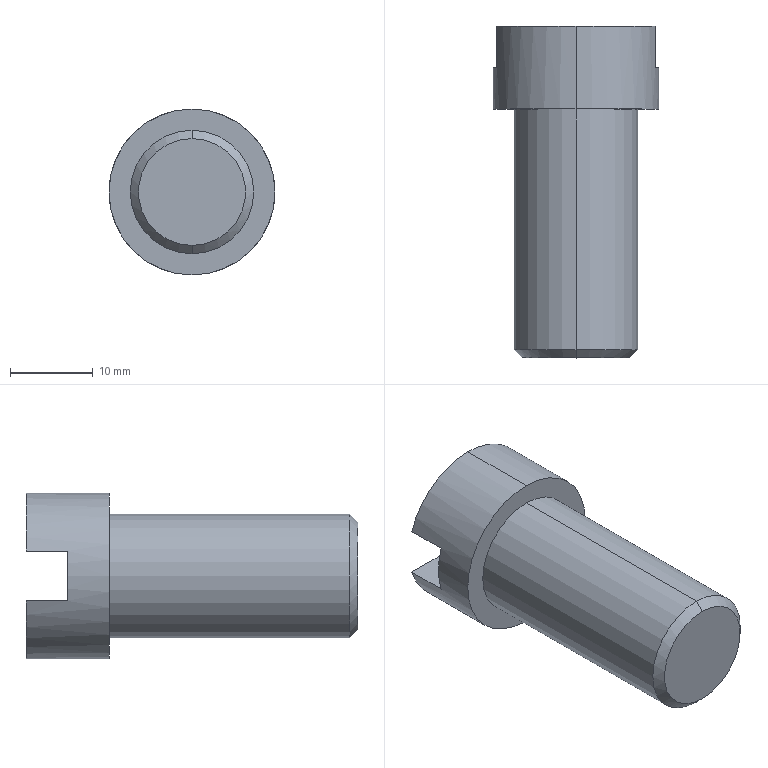Part | SolidWorks | features ICE 2, Chamfer 1, Extrusion 1 | 1 solid | 13 faces | box 20 x 40 x 20 mm | volume 7759 mm3 | plane 7 | cylinder 4 | cone 2 | commonest cylinder face diameters 14.9 x2 20 x2
STEP:
#1=CARTESIAN_POINT('',(0.,-30.,-6.45));
#2=VERTEX_POINT('',#1);
#3=CARTESIAN_POINT('',(0.,-30.,6.45));
#4=VERTEX_POINT('',#3);
#5=CARTESIAN_POINT('',(0.,-30.,0.));
#6=DIRECTION('',(0.,-1.,0.));
#7=DIRECTION('',(0.,0.,1.));
#8=AXIS2_PLACEMENT_3D('',#5,#6,#7);
#9=CIRCLE('',#8,6.45);
#10=EDGE_CURVE('',#2,#4,#9,.T.);
#11=ORIENTED_EDGE('',*,*,#10,.F.);
#12=CARTESIAN_POINT('',(0.,-29.,-7.45));
#13=VERTEX_POINT('',#12);
#14=CARTESIAN_POINT('',(0.,-29.,-7.45));
#15=DIRECTION('',(0.,0.7071,-0.7071));
#16=VECTOR('',#15,1000.);
#17=LINE('',#14,#16);
#18=EDGE_CURVE('',#2,#13,#17,.T.);
#19=ORIENTED_EDGE('',*,*,#18,.T.);
#20=CARTESIAN_POINT('',(0.,-29.,7.45));
#21=VERTEX_POINT('',#20);
#22=CARTESIAN_POINT('',(0.,-29.,0.));
#23=DIRECTION('',(0.,1.,0.));
#24=DIRECTION('',(0.,0.,1.));
#25=AXIS2_PLACEMENT_3D('',#22,#23,#24);
#26=CIRCLE('',#25,7.45);
#27=EDGE_CURVE('',#21,#13,#26,.T.);
#28=ORIENTED_EDGE('',*,*,#27,.F.);
#29=CARTESIAN_POINT('',(0.,-29.,7.45));
#30=DIRECTION('',(0.,0.7071,0.7071));
#31=VECTOR('',#30,1000.);
#32=LINE('',#29,#31);
#33=EDGE_CURVE('',#4,#21,#32,.T.);
#34=ORIENTED_EDGE('',*,*,#33,.F.);
#35=EDGE_LOOP('',(#11,#19,#28,#34));
#36=FACE_OUTER_BOUND('',#35,.T.);
#37=CARTESIAN_POINT('',(0.,-29.,0.));
#38=DIRECTION('',(0.,1.,0.));
#39=DIRECTION('',(0.,0.,1.));
#40=AXIS2_PLACEMENT_3D('',#37,#38,#39);
#41=CONICAL_SURFACE('',#40,7.45,0.7854);
#42=ADVANCED_FACE('',(#36),#41,.T.);
#43=ORIENTED_EDGE('',*,*,#27,.T.);
#44=CARTESIAN_POINT('',(0.,0.,-7.45));
#45=VERTEX_POINT('',#44);
#46=CARTESIAN_POINT('',(0.,-30.,-7.45));
#47=DIRECTION('',(0.,1.,0.));
#48=VECTOR('',#47,1000.);
#49=LINE('',#46,#48);
#50=EDGE_CURVE('',#13,#45,#49,.T.);
#51=ORIENTED_EDGE('',*,*,#50,.T.);
#52=CARTESIAN_POINT('',(0.,0.,7.45));
#53=VERTEX_POINT('',#52);
#54=CARTESIAN_POINT('',(0.,0.,0.));
#55=DIRECTION('',(0.,1.,0.));
#56=DIRECTION('',(0.,0.,1.));
#57=AXIS2_PLACEMENT_3D('',#54,#55,#56);
#58=CIRCLE('',#57,7.45);
#59=EDGE_CURVE('',#53,#45,#58,.T.);
#60=ORIENTED_EDGE('',*,*,#59,.F.);
#61=CARTESIAN_POINT('',(0.,-30.,7.45));
#62=DIRECTION('',(0.,1.,0.));
#63=VECTOR('',#62,1000.);
#64=LINE('',#61,#63);
#65=EDGE_CURVE('',#21,#53,#64,.T.);
#66=ORIENTED_EDGE('',*,*,#65,.F.);
#67=EDGE_LOOP('',(#43,#51,#60,#66));
#68=FACE_OUTER_BOUND('',#67,.T.);
#69=CARTESIAN_POINT('',(0.,-30.,0.));
#70=DIRECTION('',(0.,1.,0.));
#71=DIRECTION('',(0.,0.,1.));
#72=AXIS2_PLACEMENT_3D('',#69,#70,#71);
#73=CYLINDRICAL_SURFACE('',#72,7.45);
#74=ADVANCED_FACE('',(#68),#73,.T.);
#75=CARTESIAN_POINT('',(0.,10.,10.));
#76=VERTEX_POINT('',#75);
#77=CARTESIAN_POINT('',(9.539,10.,3.));
#78=VERTEX_POINT('',#77);
#79=CARTESIAN_POINT('',(0.,10.,0.));
#80=DIRECTION('',(0.,1.,0.));
#81=DIRECTION('',(0.,0.,1.));
#82=AXIS2_PLACEMENT_3D('',#79,#80,#81);
#83=CIRCLE('',#82,10.);
#84=EDGE_CURVE('',#76,#78,#83,.T.);
#85=ORIENTED_EDGE('',*,*,#84,.F.);
#86=CARTESIAN_POINT('',(0.,0.,10.));
#87=VERTEX_POINT('',#86);
#88=CARTESIAN_POINT('',(0.,10.,10.));
#89=DIRECTION('',(0.,-1.,0.));
#90=VECTOR('',#89,1000.);
#91=LINE('',#88,#90);
#92=EDGE_CURVE('',#76,#87,#91,.T.);
#93=ORIENTED_EDGE('',*,*,#92,.T.);
#94=CARTESIAN_POINT('',(0.,0.,-10.));
#95=VERTEX_POINT('',#94);
#96=CARTESIAN_POINT('',(0.,0.,0.));
#97=DIRECTION('',(0.,1.,0.));
#98=DIRECTION('',(0.,0.,1.));
#99=AXIS2_PLACEMENT_3D('',#96,#97,#98);
#100=CIRCLE('',#99,10.);
#101=EDGE_CURVE('',#87,#95,#100,.T.);
#102=ORIENTED_EDGE('',*,*,#101,.T.);
#103=CARTESIAN_POINT('',(0.,10.,-10.));
#104=VERTEX_POINT('',#103);
#105=CARTESIAN_POINT('',(0.,10.,-10.));
#106=DIRECTION('',(0.,-1.,0.));
#107=VECTOR('',#106,1000.);
#108=LINE('',#105,#107);
#109=EDGE_CURVE('',#104,#95,#108,.T.);
#110=ORIENTED_EDGE('',*,*,#109,.F.);
#111=CARTESIAN_POINT('',(9.539,10.,-3.));
#112=VERTEX_POINT('',#111);
#113=CARTESIAN_POINT('',(0.,10.,0.));
#114=DIRECTION('',(0.,1.,0.));
#115=DIRECTION('',(0.,0.,1.));
#116=AXIS2_PLACEMENT_3D('',#113,#114,#115);
#117=CIRCLE('',#116,10.);
#118=EDGE_CURVE('',#112,#104,#117,.T.);
#119=ORIENTED_EDGE('',*,*,#118,.F.);
#120=CARTESIAN_POINT('',(9.539,5.,-3.));
#121=VERTEX_POINT('',#120);
#122=CARTESIAN_POINT('',(9.539,10.,-3.));
#123=DIRECTION('',(0.,1.,0.));
#124=VECTOR('',#123,1000.);
#125=LINE('',#122,#124);
#126=EDGE_CURVE('',#121,#112,#125,.T.);
#127=ORIENTED_EDGE('',*,*,#126,.F.);
#128=CARTESIAN_POINT('',(9.539,5.,3.));
#129=VERTEX_POINT('',#128);
#130=CARTESIAN_POINT('',(0.,5.,0.));
#131=DIRECTION('',(0.,-1.,0.));
#132=DIRECTION('',(0.,0.,-1.));
#133=AXIS2_PLACEMENT_3D('',#130,#131,#132);
#134=CIRCLE('',#133,10.);
#135=EDGE_CURVE('',#121,#129,#134,.T.);
#136=ORIENTED_EDGE('',*,*,#135,.T.);
#137=CARTESIAN_POINT('',(9.539,10.,3.));
#138=DIRECTION('',(0.,1.,0.));
#139=VECTOR('',#138,1000.);
#140=LINE('',#137,#139);
#141=EDGE_CURVE('',#129,#78,#140,.T.);
#142=ORIENTED_EDGE('',*,*,#141,.T.);
#143=EDGE_LOOP('',(#85,#93,#102,#110,#119,#127,#136,#142));
#144=FACE_OUTER_BOUND('',#143,.T.);
#145=CARTESIAN_POINT('',(0.,10.,0.));
#146=DIRECTION('',(0.,-1.,0.));
#147=DIRECTION('',(0.,0.,-1.));
#148=AXIS2_PLACEMENT_3D('',#145,#146,#147);
#149=CYLINDRICAL_SURFACE('',#148,10.);
#150=ADVANCED_FACE('',(#144),#149,.T.);
#151=ORIENTED_EDGE('',*,*,#92,.F.);
#152=CARTESIAN_POINT('',(-9.539,10.,3.));
#153=VERTEX_POINT('',#152);
#154=CARTESIAN_POINT('',(0.,10.,0.));
#155=DIRECTION('',(0.,1.,0.));
#156=DIRECTION('',(0.,0.,1.));
#157=AXIS2_PLACEMENT_3D('',#154,#155,#156);
#158=CIRCLE('',#157,10.);
#159=EDGE_CURVE('',#153,#76,#158,.T.);
#160=ORIENTED_EDGE('',*,*,#159,.F.);
#161=CARTESIAN_POINT('',(-9.539,5.,3.));
#162=VERTEX_POINT('',#161);
#163=CARTESIAN_POINT('',(-9.539,10.,3.));
#164=DIRECTION('',(0.,-1.,0.));
#165=VECTOR('',#164,1000.);
#166=LINE('',#163,#165);
#167=EDGE_CURVE('',#153,#162,#166,.T.);
#168=ORIENTED_EDGE('',*,*,#167,.T.);
#169=CARTESIAN_POINT('',(-9.539,5.,-3.));
#170=VERTEX_POINT('',#169);
#171=CARTESIAN_POINT('',(0.,5.,0.));
#172=DIRECTION('',(0.,-1.,0.));
#173=DIRECTION('',(0.,0.,-1.));
#174=AXIS2_PLACEMENT_3D('',#171,#172,#173);
#175=CIRCLE('',#174,10.);
#176=EDGE_CURVE('',#162,#170,#175,.T.);
#177=ORIENTED_EDGE('',*,*,#176,.T.);
#178=CARTESIAN_POINT('',(-9.539,10.,-3.));
#179=VERTEX_POINT('',#178);
#180=CARTESIAN_POINT('',(-9.539,10.,-3.));
#181=DIRECTION('',(0.,-1.,0.));
#182=VECTOR('',#181,1000.);
#183=LINE('',#180,#182);
#184=EDGE_CURVE('',#179,#170,#183,.T.);
#185=ORIENTED_EDGE('',*,*,#184,.F.);
#186=CARTESIAN_POINT('',(0.,10.,0.));
#187=DIRECTION('',(0.,1.,0.));
#188=DIRECTION('',(0.,0.,1.));
#189=AXIS2_PLACEMENT_3D('',#186,#187,#188);
#190=CIRCLE('',#189,10.);
#191=EDGE_CURVE('',#104,#179,#190,.T.);
#192=ORIENTED_EDGE('',*,*,#191,.F.);
#193=ORIENTED_EDGE('',*,*,#109,.T.);
#194=CARTESIAN_POINT('',(0.,0.,0.));
#195=DIRECTION('',(0.,1.,0.));
#196=DIRECTION('',(0.,0.,1.));
#197=AXIS2_PLACEMENT_3D('',#194,#195,#196);
#198=CIRCLE('',#197,10.);
#199=EDGE_CURVE('',#95,#87,#198,.T.);
#200=ORIENTED_EDGE('',*,*,#199,.T.);
#201=EDGE_LOOP('',(#151,#160,#168,#177,#185,#192,#193,#200));
#202=FACE_OUTER_BOUND('',#201,.T.);
#203=CARTESIAN_POINT('',(0.,10.,0.));
#204=DIRECTION('',(0.,-1.,0.));
#205=DIRECTION('',(0.,0.,-1.));
#206=AXIS2_PLACEMENT_3D('',#203,#204,#205);
#207=CYLINDRICAL_SURFACE('',#206,10.);
#208=ADVANCED_FACE('',(#202),#207,.T.);
#209=ORIENTED_EDGE('',*,*,#118,.T.);
#210=ORIENTED_EDGE('',*,*,#191,.T.);
#211=CARTESIAN_POINT('',(0.,10.,-3.));
#212=DIRECTION('',(1.,0.,0.));
#213=VECTOR('',#212,1000.);
#214=LINE('',#211,#213);
#215=EDGE_CURVE('',#179,#112,#214,.T.);
#216=ORIENTED_EDGE('',*,*,#215,.T.);
#217=EDGE_LOOP('',(#209,#210,#216));
#218=FACE_OUTER_BOUND('',#217,.T.);
#219=CARTESIAN_POINT('',(0.,10.,0.));
#220=DIRECTION('',(0.,1.,0.));
#221=DIRECTION('',(0.,0.,1.));
#222=AXIS2_PLACEMENT_3D('',#219,#220,#221);
#223=PLANE('',#222);
#224=ADVANCED_FACE('',(#218),#223,.T.);
#225=ORIENTED_EDGE('',*,*,#50,.F.);
#226=CARTESIAN_POINT('',(0.,-29.,0.));
#227=DIRECTION('',(0.,1.,0.));
#228=DIRECTION('',(0.,0.,1.));
#229=AXIS2_PLACEMENT_3D('',#226,#227,#228);
#230=CIRCLE('',#229,7.45);
#231=EDGE_CURVE('',#13,#21,#230,.T.);
#232=ORIENTED_EDGE('',*,*,#231,.T.);
#233=ORIENTED_EDGE('',*,*,#65,.T.);
#234=CARTESIAN_POINT('',(0.,0.,0.));
#235=DIRECTION('',(0.,1.,0.));
#236=DIRECTION('',(0.,0.,1.));
#237=AXIS2_PLACEMENT_3D('',#234,#235,#236);
#238=CIRCLE('',#237,7.45);
#239=EDGE_CURVE('',#45,#53,#238,.T.);
#240=ORIENTED_EDGE('',*,*,#239,.F.);
#241=EDGE_LOOP('',(#225,#232,#233,#240));
#242=FACE_OUTER_BOUND('',#241,.T.);
#243=CARTESIAN_POINT('',(0.,-30.,0.));
#244=DIRECTION('',(0.,1.,0.));
#245=DIRECTION('',(0.,0.,1.));
#246=AXIS2_PLACEMENT_3D('',#243,#244,#245);
#247=CYLINDRICAL_SURFACE('',#246,7.45);
#248=ADVANCED_FACE('',(#242),#247,.T.);
#249=CARTESIAN_POINT('',(0.,-30.,0.));
#250=DIRECTION('',(0.,-1.,0.));
#251=DIRECTION('',(0.,0.,1.));
#252=AXIS2_PLACEMENT_3D('',#249,#250,#251);
#253=CIRCLE('',#252,6.45);
#254=EDGE_CURVE('',#4,#2,#253,.T.);
#255=ORIENTED_EDGE('',*,*,#254,.T.);
#256=ORIENTED_EDGE('',*,*,#10,.T.);
#257=EDGE_LOOP('',(#255,#256));
#258=FACE_OUTER_BOUND('',#257,.T.);
#259=CARTESIAN_POINT('',(0.,-30.,0.));
#260=DIRECTION('',(0.,1.,0.));
#261=DIRECTION('',(0.,0.,1.));
#262=AXIS2_PLACEMENT_3D('',#259,#260,#261);
#263=PLANE('',#262);
#264=ADVANCED_FACE('',(#258),#263,.F.);
#265=CARTESIAN_POINT('',(0.,10.,3.));
#266=DIRECTION('',(1.,0.,0.));
#267=VECTOR('',#266,1000.);
#268=LINE('',#265,#267);
#269=EDGE_CURVE('',#153,#78,#268,.T.);
#270=ORIENTED_EDGE('',*,*,#269,.F.);
#271=ORIENTED_EDGE('',*,*,#159,.T.);
#272=ORIENTED_EDGE('',*,*,#84,.T.);
#273=EDGE_LOOP('',(#270,#271,#272));
#274=FACE_OUTER_BOUND('',#273,.T.);
#275=CARTESIAN_POINT('',(0.,10.,0.));
#276=DIRECTION('',(0.,1.,0.));
#277=DIRECTION('',(0.,0.,1.));
#278=AXIS2_PLACEMENT_3D('',#275,#276,#277);
#279=PLANE('',#278);
#280=ADVANCED_FACE('',(#274),#279,.T.);
#281=ORIENTED_EDGE('',*,*,#59,.T.);
#282=ORIENTED_EDGE('',*,*,#239,.T.);
#283=EDGE_LOOP('',(#281,#282));
#284=FACE_BOUND('',#283,.T.);
#285=ORIENTED_EDGE('',*,*,#199,.F.);
#286=ORIENTED_EDGE('',*,*,#101,.F.);
#287=EDGE_LOOP('',(#285,#286));
#288=FACE_OUTER_BOUND('',#287,.T.);
#289=CARTESIAN_POINT('',(0.,0.,0.));
#290=DIRECTION('',(0.,1.,0.));
#291=DIRECTION('',(0.,0.,1.));
#292=AXIS2_PLACEMENT_3D('',#289,#290,#291);
#293=PLANE('',#292);
#294=ADVANCED_FACE('',(#284,#288),#293,.F.);
#295=CARTESIAN_POINT('',(-25.,5.,-3.));
#296=DIRECTION('',(1.,0.,0.));
#297=VECTOR('',#296,1000.);
#298=LINE('',#295,#297);
#299=EDGE_CURVE('',#170,#121,#298,.T.);
#300=ORIENTED_EDGE('',*,*,#299,.F.);
#301=ORIENTED_EDGE('',*,*,#176,.F.);
#302=CARTESIAN_POINT('',(-25.,5.,3.));
#303=DIRECTION('',(1.,0.,0.));
#304=VECTOR('',#303,1000.);
#305=LINE('',#302,#304);
#306=EDGE_CURVE('',#162,#129,#305,.T.);
#307=ORIENTED_EDGE('',*,*,#306,.T.);
#308=ORIENTED_EDGE('',*,*,#135,.F.);
#309=EDGE_LOOP('',(#300,#301,#307,#308));
#310=FACE_OUTER_BOUND('',#309,.T.);
#311=CARTESIAN_POINT('',(0.,5.,0.));
#312=DIRECTION('',(0.,-1.,0.));
#313=DIRECTION('',(0.,0.,-1.));
#314=AXIS2_PLACEMENT_3D('',#311,#312,#313);
#315=PLANE('',#314);
#316=ADVANCED_FACE('',(#310),#315,.F.);
#317=ORIENTED_EDGE('',*,*,#184,.T.);
#318=ORIENTED_EDGE('',*,*,#299,.T.);
#319=ORIENTED_EDGE('',*,*,#126,.T.);
#320=ORIENTED_EDGE('',*,*,#215,.F.);
#321=EDGE_LOOP('',(#317,#318,#319,#320));
#322=FACE_OUTER_BOUND('',#321,.T.);
#323=CARTESIAN_POINT('',(-25.,5.,-3.));
#324=DIRECTION('',(0.,0.,1.));
#325=DIRECTION('',(1.,0.,0.));
#326=AXIS2_PLACEMENT_3D('',#323,#324,#325);
#327=PLANE('',#326);
#328=ADVANCED_FACE('',(#322),#327,.T.);
#329=ORIENTED_EDGE('',*,*,#269,.T.);
#330=ORIENTED_EDGE('',*,*,#141,.F.);
#331=ORIENTED_EDGE('',*,*,#306,.F.);
#332=ORIENTED_EDGE('',*,*,#167,.F.);
#333=EDGE_LOOP('',(#329,#330,#331,#332));
#334=FACE_OUTER_BOUND('',#333,.T.);
#335=CARTESIAN_POINT('',(-25.,5.,3.));
#336=DIRECTION('',(0.,0.,1.));
#337=DIRECTION('',(1.,0.,0.));
#338=AXIS2_PLACEMENT_3D('',#335,#336,#337);
#339=PLANE('',#338);
#340=ADVANCED_FACE('',(#334),#339,.F.);
#341=ORIENTED_EDGE('',*,*,#18,.F.);
#342=ORIENTED_EDGE('',*,*,#254,.F.);
#343=ORIENTED_EDGE('',*,*,#33,.T.);
#344=ORIENTED_EDGE('',*,*,#231,.F.);
#345=EDGE_LOOP('',(#341,#342,#343,#344));
#346=FACE_OUTER_BOUND('',#345,.T.);
#347=CARTESIAN_POINT('',(0.,-29.,0.));
#348=DIRECTION('',(0.,1.,0.));
#349=DIRECTION('',(0.,0.,1.));
#350=AXIS2_PLACEMENT_3D('',#347,#348,#349);
#351=CONICAL_SURFACE('',#350,7.45,0.7854);
#352=ADVANCED_FACE('',(#346),#351,.T.);
#353=CLOSED_SHELL('',(#42,#74,#150,#208,#224,#248,#264,#280,#294,#316,#328,#340,#352));
#354=MANIFOLD_SOLID_BREP('',#353);
#355=CARTESIAN_POINT('',(0.,0.,0.));
#356=DIRECTION('',(0.,0.,1.));
#357=DIRECTION('',(1.,0.,0.));
#358=AXIS2_PLACEMENT_3D('',#355,#356,#357);
#359=(LENGTH_UNIT()NAMED_UNIT(*)SI_UNIT(.MILLI.,.METRE.));
#360=UNCERTAINTY_MEASURE_WITH_UNIT(LENGTH_MEASURE(0.00001),#359,'','');
#361=(NAMED_UNIT(*)PLANE_ANGLE_UNIT()SI_UNIT($,.RADIAN.));
#362=(NAMED_UNIT(*)SI_UNIT($,.STERADIAN.)SOLID_ANGLE_UNIT());
#363=(GEOMETRIC_REPRESENTATION_CONTEXT(3)GLOBAL_UNCERTAINTY_ASSIGNED_CONTEXT((#360))GLOBAL_UNIT_ASSIGNED_CONTEXT((#359,#361,#362))REPRESENTATION_CONTEXT('',''));
#364=ADVANCED_BREP_SHAPE_REPRESENTATION('',(#354,#358),#363);